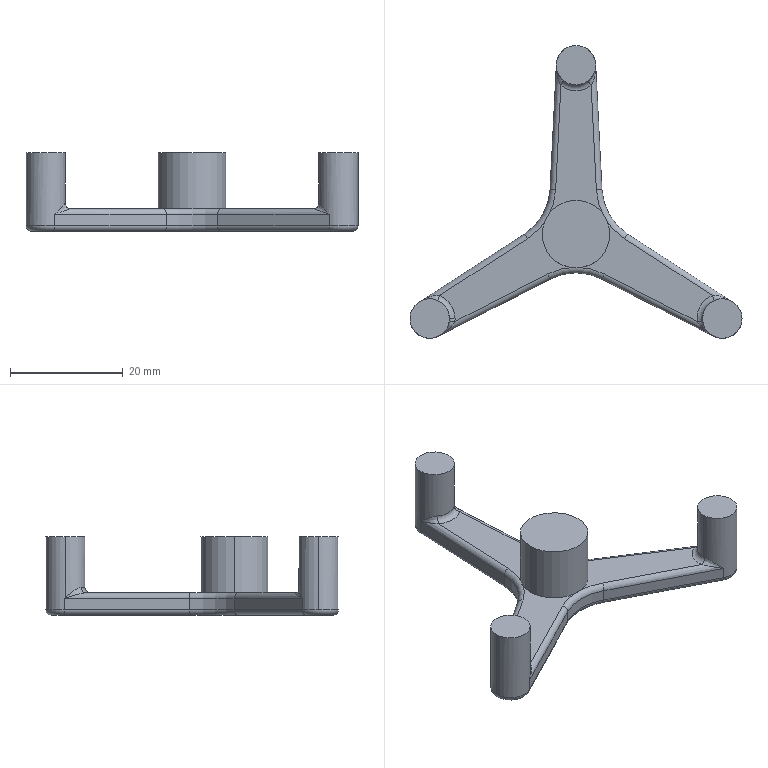Part | SolidWorks | features Boss 1, Extrusion 1, Fillet 1 | 2 solids | 56 faces | box 58.962 x 52 x 14 mm | volume 5388 mm3 | cylinder 23 | torus 14 | plane 13 | spline 6 | commonest cylinder face diameters 2 x12 7 x6 20 x3 12 x2